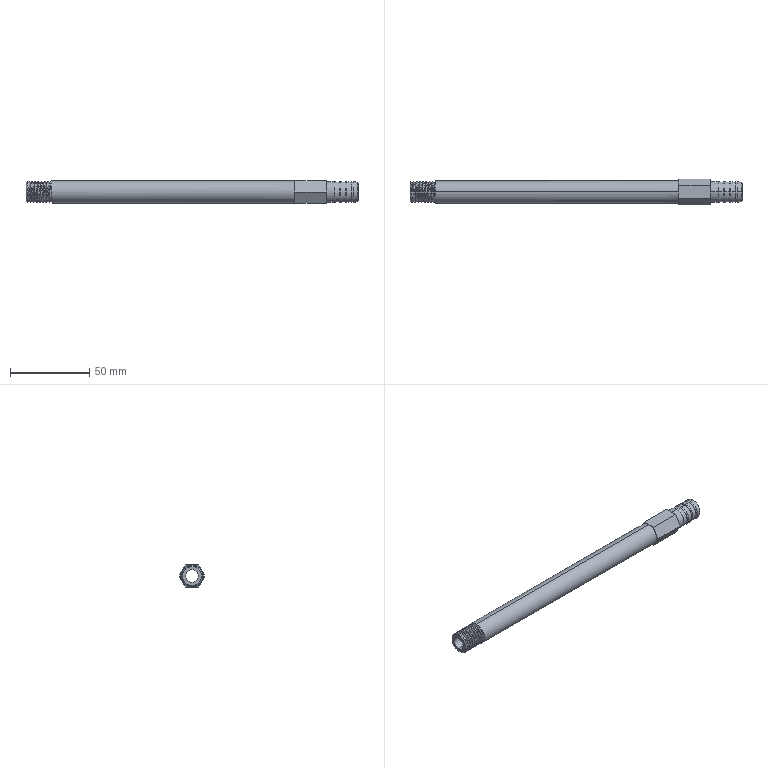Part | SolidWorks | features BaseBody 1 | 1 solid | 82 faces | box 210 x 16.166 x 14 mm | volume 21077 mm3 | cylinder 45 | plane 21 | cone 14 | spline 2 | commonest cylinder face diameters 13.6 x17 11.6 x16 13 x8 8 x2 14 x2